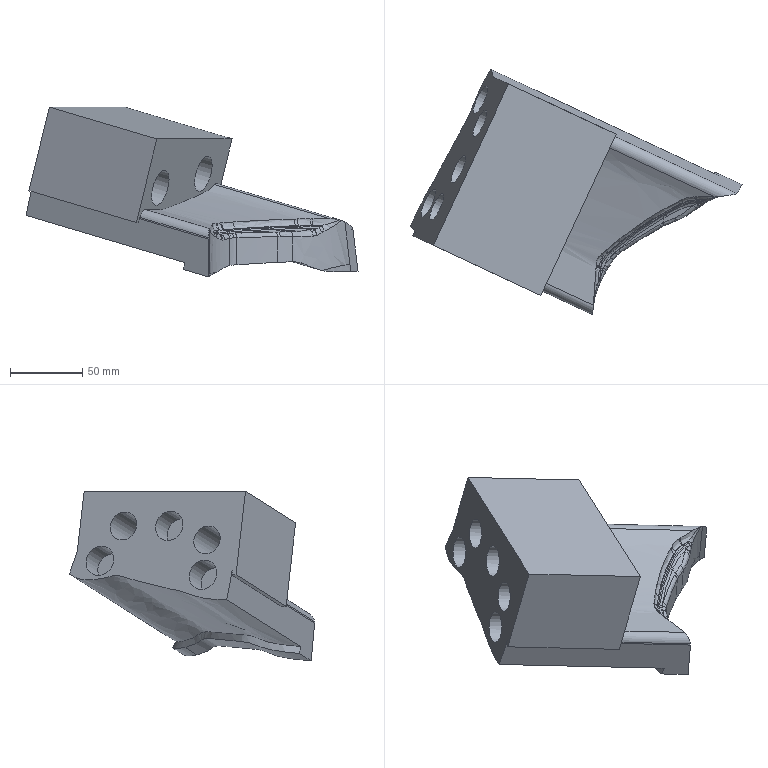Part | NX | features solid 2 | 1 solid | 100 faces | box 229.886 x 169.717 x 117.575 mm | volume 836204 mm3 | spline 78 | plane 13 | cylinder 9 | commonest cylinder face diameters 21 x3 12 x2 20 x2 25 x2